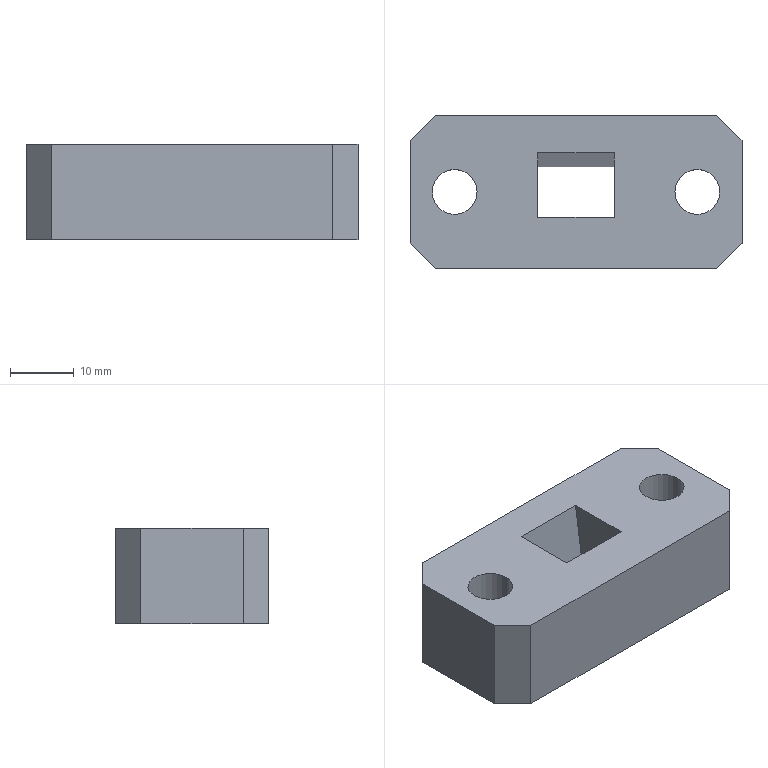Part | Creo | 1 solid | 145 faces | box 52 x 24 x 15 mm | volume 14476 mm3 | other 89 | plane 47 | cylinder 9 | commonest cylinder face diameters 7 x4 11 x4 17.925 x1